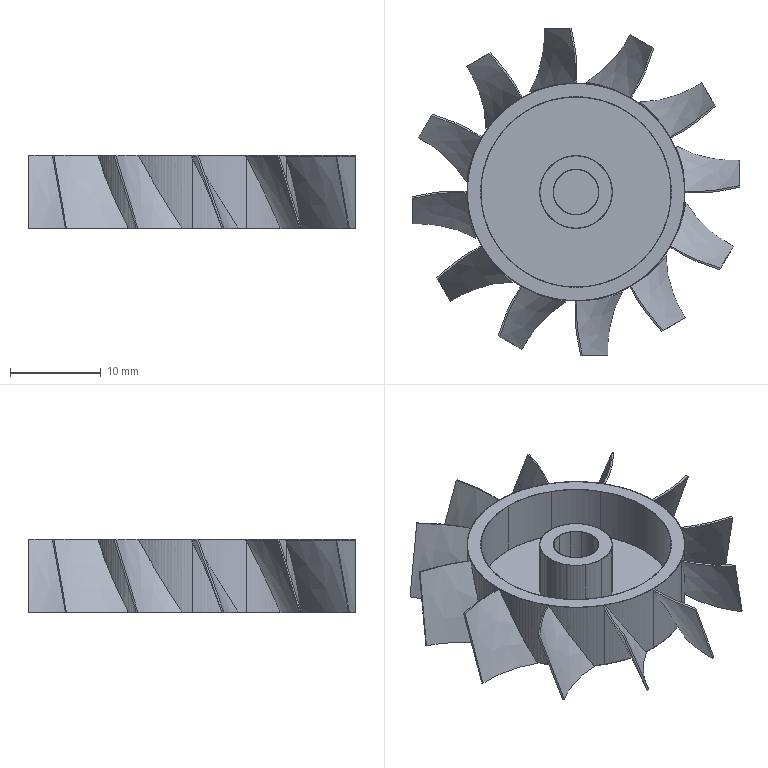Part | SolidWorks | features BlendRefSurface 1, CirPattern 1, RefCurve 1, Revolution 1, Thicken 1 | 12 solids | 228 faces | box 36.047 x 36.047 x 8.091 mm | volume 20832 mm3 | cylinder 96 | spline 72 | plane 60 | commonest cylinder face diameters 5 x24 8 x24 21 x24 24 x24